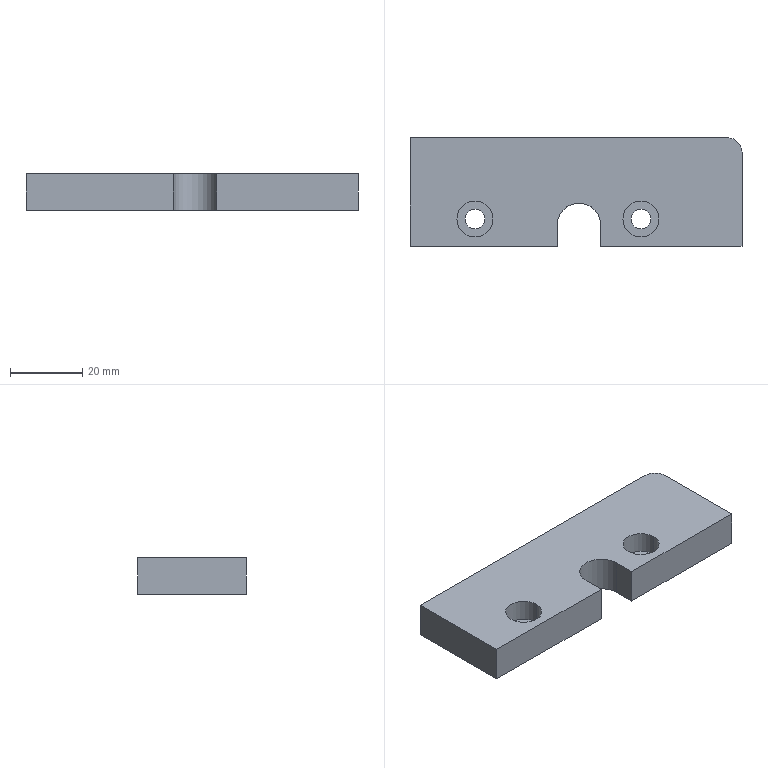Part | STEP file | ASND-0110-TCTF01-57-1 | 1 solid | 22 faces | box 92 x 30 x 10 mm | volume 25160 mm3 | cylinder 11 | plane 11 | commonest cylinder face diameters 5.5 x4 10 x4 8 x2 12 x1